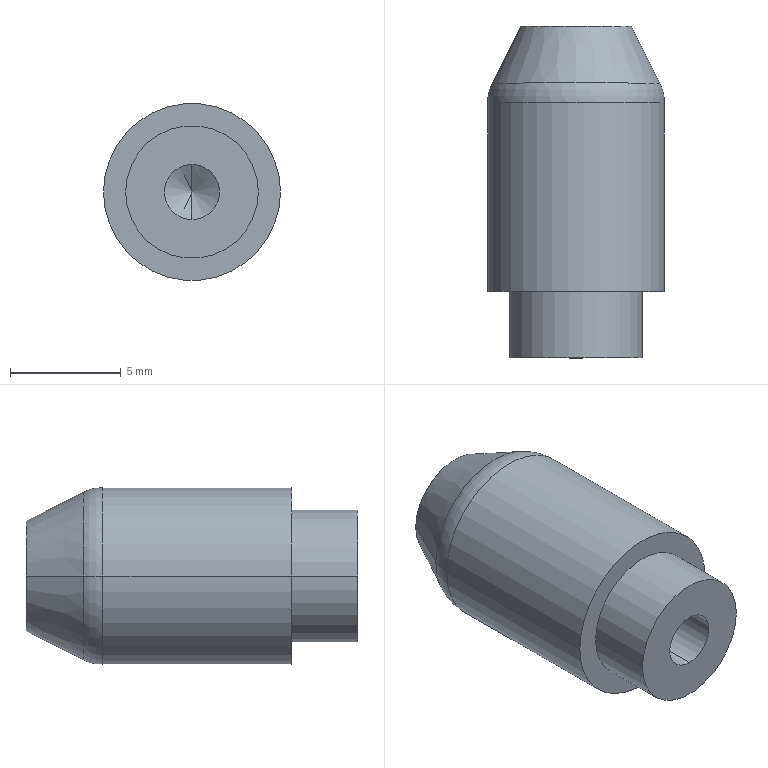Part | SolidWorks | features Fillet 1, HoleWzd 1, Revolution 1 | 1 solid | 15 faces | box 8 x 15 x 8 mm | volume 587.79 mm3 | cylinder 6 | cone 4 | plane 3 | torus 2 | commonest cylinder face diameters 2.5 x2 6 x2 8 x2
STEP:
#1=CARTESIAN_POINT('',(4.,11.528,0.));
#2=VERTEX_POINT('',#1);
#3=CARTESIAN_POINT('',(-4.,11.528,0.));
#4=VERTEX_POINT('',#3);
#5=CARTESIAN_POINT('',(0.,11.528,0.));
#6=DIRECTION('',(0.,-1.,0.));
#7=DIRECTION('',(-1.,0.,0.));
#8=AXIS2_PLACEMENT_3D('',#5,#6,#7);
#9=CIRCLE('',#8,4.);
#10=EDGE_CURVE('',#2,#4,#9,.T.);
#11=ORIENTED_EDGE('',*,*,#10,.F.);
#12=CARTESIAN_POINT('',(3.789,12.422,0.));
#13=VERTEX_POINT('',#12);
#14=CARTESIAN_POINT('',(2.,11.528,0.));
#15=DIRECTION('',(0.,0.,1.));
#16=DIRECTION('',(1.,0.,0.));
#17=AXIS2_PLACEMENT_3D('',#14,#15,#16);
#18=CIRCLE('',#17,2.);
#19=EDGE_CURVE('',#2,#13,#18,.T.);
#20=ORIENTED_EDGE('',*,*,#19,.T.);
#21=CARTESIAN_POINT('',(-3.789,12.422,0.));
#22=VERTEX_POINT('',#21);
#23=CARTESIAN_POINT('',(0.,12.422,0.));
#24=DIRECTION('',(0.,1.,0.));
#25=DIRECTION('',(-1.,0.,0.));
#26=AXIS2_PLACEMENT_3D('',#23,#24,#25);
#27=CIRCLE('',#26,3.789);
#28=EDGE_CURVE('',#22,#13,#27,.T.);
#29=ORIENTED_EDGE('',*,*,#28,.F.);
#30=CARTESIAN_POINT('',(-2.,11.528,0.));
#31=DIRECTION('',(0.,0.,-1.));
#32=DIRECTION('',(-1.,0.,0.));
#33=AXIS2_PLACEMENT_3D('',#30,#31,#32);
#34=CIRCLE('',#33,2.);
#35=EDGE_CURVE('',#4,#22,#34,.T.);
#36=ORIENTED_EDGE('',*,*,#35,.F.);
#37=EDGE_LOOP('',(#11,#20,#29,#36));
#38=FACE_OUTER_BOUND('',#37,.T.);
#39=CARTESIAN_POINT('',(0.,11.528,0.));
#40=DIRECTION('',(0.,1.,0.));
#41=DIRECTION('',(-1.,0.,0.));
#42=AXIS2_PLACEMENT_3D('',#39,#40,#41);
#43=TOROIDAL_SURFACE('',#42,2.,2.);
#44=ADVANCED_FACE('',(#38),#43,.T.);
#45=CARTESIAN_POINT('',(0.,10.,1.25));
#46=VERTEX_POINT('',#45);
#47=CARTESIAN_POINT('',(0.,10.,-1.25));
#48=VERTEX_POINT('',#47);
#49=CARTESIAN_POINT('',(0.,10.,0.));
#50=DIRECTION('',(0.,-1.,0.));
#51=DIRECTION('',(0.,0.,-1.));
#52=AXIS2_PLACEMENT_3D('',#49,#50,#51);
#53=CIRCLE('',#52,1.25);
#54=EDGE_CURVE('',#46,#48,#53,.T.);
#55=ORIENTED_EDGE('',*,*,#54,.F.);
#56=CARTESIAN_POINT('',(0.,0.,1.25));
#57=VERTEX_POINT('',#56);
#58=CARTESIAN_POINT('',(0.,0.,1.25));
#59=DIRECTION('',(0.,-1.,0.));
#60=VECTOR('',#59,1000.);
#61=LINE('',#58,#60);
#62=EDGE_CURVE('',#46,#57,#61,.T.);
#63=ORIENTED_EDGE('',*,*,#62,.T.);
#64=CARTESIAN_POINT('',(0.,0.,-1.25));
#65=VERTEX_POINT('',#64);
#66=CARTESIAN_POINT('',(0.,0.,0.));
#67=DIRECTION('',(0.,-1.,0.));
#68=DIRECTION('',(0.,0.,-1.));
#69=AXIS2_PLACEMENT_3D('',#66,#67,#68);
#70=CIRCLE('',#69,1.25);
#71=EDGE_CURVE('',#57,#65,#70,.T.);
#72=ORIENTED_EDGE('',*,*,#71,.T.);
#73=CARTESIAN_POINT('',(0.,0.,-1.25));
#74=DIRECTION('',(0.,-1.,0.));
#75=VECTOR('',#74,1000.);
#76=LINE('',#73,#75);
#77=EDGE_CURVE('',#48,#65,#76,.T.);
#78=ORIENTED_EDGE('',*,*,#77,.F.);
#79=EDGE_LOOP('',(#55,#63,#72,#78));
#80=FACE_OUTER_BOUND('',#79,.T.);
#81=CARTESIAN_POINT('',(0.,0.,0.));
#82=DIRECTION('',(0.,-1.,0.));
#83=DIRECTION('',(0.,0.,-1.));
#84=AXIS2_PLACEMENT_3D('',#81,#82,#83);
#85=CYLINDRICAL_SURFACE('',#84,1.25);
#86=ADVANCED_FACE('',(#80),#85,.F.);
#87=CARTESIAN_POINT('',(0.,10.751,0.));
#88=VERTEX_POINT('',#87);
#89=CARTESIAN_POINT('',(0.,10.,-1.25));
#90=DIRECTION('',(0.,-0.515,-0.8572));
#91=VECTOR('',#90,1000.);
#92=LINE('',#89,#91);
#93=EDGE_CURVE('',#88,#48,#92,.T.);
#94=ORIENTED_EDGE('',*,*,#93,.F.);
#95=CARTESIAN_POINT('',(0.,10.,1.25));
#96=DIRECTION('',(0.,-0.515,0.8572));
#97=VECTOR('',#96,1000.);
#98=LINE('',#95,#97);
#99=EDGE_CURVE('',#88,#46,#98,.T.);
#100=ORIENTED_EDGE('',*,*,#99,.T.);
#101=ORIENTED_EDGE('',*,*,#54,.T.);
#102=EDGE_LOOP('',(#94,#100,#101));
#103=FACE_OUTER_BOUND('',#102,.T.);
#104=CARTESIAN_POINT('',(0.,10.,0.));
#105=DIRECTION('',(0.,-1.,0.));
#106=DIRECTION('',(0.,0.,-1.));
#107=AXIS2_PLACEMENT_3D('',#104,#105,#106);
#108=CONICAL_SURFACE('',#107,1.25,1.03);
#109=ADVANCED_FACE('',(#103),#108,.F.);
#110=CARTESIAN_POINT('',(3.,3.,0.));
#111=VERTEX_POINT('',#110);
#112=CARTESIAN_POINT('',(-3.,3.,0.));
#113=VERTEX_POINT('',#112);
#114=CARTESIAN_POINT('',(0.,3.,0.));
#115=DIRECTION('',(0.,-1.,0.));
#116=DIRECTION('',(1.,0.,0.));
#117=AXIS2_PLACEMENT_3D('',#114,#115,#116);
#118=CIRCLE('',#117,3.);
#119=EDGE_CURVE('',#111,#113,#118,.T.);
#120=ORIENTED_EDGE('',*,*,#119,.T.);
#121=CARTESIAN_POINT('',(-3.,0.,0.));
#122=VERTEX_POINT('',#121);
#123=CARTESIAN_POINT('',(-3.,0.,0.));
#124=DIRECTION('',(0.,-1.,0.));
#125=VECTOR('',#124,1000.);
#126=LINE('',#123,#125);
#127=EDGE_CURVE('',#113,#122,#126,.T.);
#128=ORIENTED_EDGE('',*,*,#127,.T.);
#129=CARTESIAN_POINT('',(3.,0.,0.));
#130=VERTEX_POINT('',#129);
#131=CARTESIAN_POINT('',(0.,0.,0.));
#132=DIRECTION('',(0.,-1.,0.));
#133=DIRECTION('',(1.,0.,0.));
#134=AXIS2_PLACEMENT_3D('',#131,#132,#133);
#135=CIRCLE('',#134,3.);
#136=EDGE_CURVE('',#130,#122,#135,.T.);
#137=ORIENTED_EDGE('',*,*,#136,.F.);
#138=CARTESIAN_POINT('',(3.,0.,0.));
#139=DIRECTION('',(0.,-1.,0.));
#140=VECTOR('',#139,1000.);
#141=LINE('',#138,#140);
#142=EDGE_CURVE('',#111,#130,#141,.T.);
#143=ORIENTED_EDGE('',*,*,#142,.F.);
#144=EDGE_LOOP('',(#120,#128,#137,#143));
#145=FACE_OUTER_BOUND('',#144,.T.);
#146=CARTESIAN_POINT('',(0.,0.,0.));
#147=DIRECTION('',(0.,-1.,0.));
#148=DIRECTION('',(1.,0.,0.));
#149=AXIS2_PLACEMENT_3D('',#146,#147,#148);
#150=CYLINDRICAL_SURFACE('',#149,3.);
#151=ADVANCED_FACE('',(#145),#150,.T.);
#152=ORIENTED_EDGE('',*,*,#10,.T.);
#153=CARTESIAN_POINT('',(-4.,3.,0.));
#154=VERTEX_POINT('',#153);
#155=CARTESIAN_POINT('',(-4.,0.,0.));
#156=DIRECTION('',(0.,-1.,0.));
#157=VECTOR('',#156,1000.);
#158=LINE('',#155,#157);
#159=EDGE_CURVE('',#4,#154,#158,.T.);
#160=ORIENTED_EDGE('',*,*,#159,.T.);
#161=CARTESIAN_POINT('',(4.,3.,0.));
#162=VERTEX_POINT('',#161);
#163=CARTESIAN_POINT('',(0.,3.,0.));
#164=DIRECTION('',(0.,-1.,0.));
#165=DIRECTION('',(1.,0.,0.));
#166=AXIS2_PLACEMENT_3D('',#163,#164,#165);
#167=CIRCLE('',#166,4.);
#168=EDGE_CURVE('',#162,#154,#167,.T.);
#169=ORIENTED_EDGE('',*,*,#168,.F.);
#170=CARTESIAN_POINT('',(4.,0.,0.));
#171=DIRECTION('',(0.,-1.,0.));
#172=VECTOR('',#171,1000.);
#173=LINE('',#170,#172);
#174=EDGE_CURVE('',#2,#162,#173,.T.);
#175=ORIENTED_EDGE('',*,*,#174,.F.);
#176=EDGE_LOOP('',(#152,#160,#169,#175));
#177=FACE_OUTER_BOUND('',#176,.T.);
#178=CARTESIAN_POINT('',(0.,0.,0.));
#179=DIRECTION('',(0.,-1.,0.));
#180=DIRECTION('',(1.,0.,0.));
#181=AXIS2_PLACEMENT_3D('',#178,#179,#180);
#182=CYLINDRICAL_SURFACE('',#181,4.);
#183=ADVANCED_FACE('',(#177),#182,.T.);
#184=CARTESIAN_POINT('',(2.5,15.,0.));
#185=VERTEX_POINT('',#184);
#186=CARTESIAN_POINT('',(-2.5,15.,0.));
#187=VERTEX_POINT('',#186);
#188=CARTESIAN_POINT('',(0.,15.,0.));
#189=DIRECTION('',(0.,-1.,0.));
#190=DIRECTION('',(1.,0.,0.));
#191=AXIS2_PLACEMENT_3D('',#188,#189,#190);
#192=CIRCLE('',#191,2.5);
#193=EDGE_CURVE('',#185,#187,#192,.T.);
#194=ORIENTED_EDGE('',*,*,#193,.T.);
#195=CARTESIAN_POINT('',(-4.,12.,0.));
#196=DIRECTION('',(-0.4472,-0.8944,0.));
#197=VECTOR('',#196,1000.);
#198=LINE('',#195,#197);
#199=EDGE_CURVE('',#187,#22,#198,.T.);
#200=ORIENTED_EDGE('',*,*,#199,.T.);
#201=ORIENTED_EDGE('',*,*,#28,.T.);
#202=CARTESIAN_POINT('',(4.,12.,0.));
#203=DIRECTION('',(0.4472,-0.8944,0.));
#204=VECTOR('',#203,1000.);
#205=LINE('',#202,#204);
#206=EDGE_CURVE('',#185,#13,#205,.T.);
#207=ORIENTED_EDGE('',*,*,#206,.F.);
#208=EDGE_LOOP('',(#194,#200,#201,#207));
#209=FACE_OUTER_BOUND('',#208,.T.);
#210=CARTESIAN_POINT('',(0.,12.,0.));
#211=DIRECTION('',(0.,-1.,0.));
#212=DIRECTION('',(1.,0.,0.));
#213=AXIS2_PLACEMENT_3D('',#210,#211,#212);
#214=CONICAL_SURFACE('',#213,4.,0.4636);
#215=ADVANCED_FACE('',(#209),#214,.T.);
#216=CARTESIAN_POINT('',(0.,0.,0.));
#217=DIRECTION('',(0.,-1.,0.));
#218=DIRECTION('',(0.,0.,-1.));
#219=AXIS2_PLACEMENT_3D('',#216,#217,#218);
#220=CIRCLE('',#219,1.25);
#221=EDGE_CURVE('',#65,#57,#220,.T.);
#222=ORIENTED_EDGE('',*,*,#221,.F.);
#223=ORIENTED_EDGE('',*,*,#71,.F.);
#224=EDGE_LOOP('',(#222,#223));
#225=FACE_BOUND('',#224,.T.);
#226=ORIENTED_EDGE('',*,*,#136,.T.);
#227=CARTESIAN_POINT('',(0.,0.,0.));
#228=DIRECTION('',(0.,-1.,0.));
#229=DIRECTION('',(1.,0.,0.));
#230=AXIS2_PLACEMENT_3D('',#227,#228,#229);
#231=CIRCLE('',#230,3.);
#232=EDGE_CURVE('',#122,#130,#231,.T.);
#233=ORIENTED_EDGE('',*,*,#232,.T.);
#234=EDGE_LOOP('',(#226,#233));
#235=FACE_OUTER_BOUND('',#234,.T.);
#236=CARTESIAN_POINT('',(3.,0.,0.));
#237=DIRECTION('',(0.,-1.,0.));
#238=DIRECTION('',(1.,0.,0.));
#239=AXIS2_PLACEMENT_3D('',#236,#237,#238);
#240=PLANE('',#239);
#241=ADVANCED_FACE('',(#225,#235),#240,.T.);
#242=ORIENTED_EDGE('',*,*,#193,.F.);
#243=CARTESIAN_POINT('',(0.,15.,0.));
#244=DIRECTION('',(0.,-1.,0.));
#245=DIRECTION('',(1.,0.,0.));
#246=AXIS2_PLACEMENT_3D('',#243,#244,#245);
#247=CIRCLE('',#246,2.5);
#248=EDGE_CURVE('',#187,#185,#247,.T.);
#249=ORIENTED_EDGE('',*,*,#248,.F.);
#250=EDGE_LOOP('',(#242,#249));
#251=FACE_OUTER_BOUND('',#250,.T.);
#252=CARTESIAN_POINT('',(0.,15.,0.));
#253=DIRECTION('',(0.,1.,0.));
#254=DIRECTION('',(-1.,0.,0.));
#255=AXIS2_PLACEMENT_3D('',#252,#253,#254);
#256=PLANE('',#255);
#257=ADVANCED_FACE('',(#251),#256,.T.);
#258=ORIENTED_EDGE('',*,*,#199,.F.);
#259=ORIENTED_EDGE('',*,*,#248,.T.);
#260=ORIENTED_EDGE('',*,*,#206,.T.);
#261=CARTESIAN_POINT('',(0.,12.422,0.));
#262=DIRECTION('',(0.,1.,0.));
#263=DIRECTION('',(-1.,0.,0.));
#264=AXIS2_PLACEMENT_3D('',#261,#262,#263);
#265=CIRCLE('',#264,3.789);
#266=EDGE_CURVE('',#13,#22,#265,.T.);
#267=ORIENTED_EDGE('',*,*,#266,.T.);
#268=EDGE_LOOP('',(#258,#259,#260,#267));
#269=FACE_OUTER_BOUND('',#268,.T.);
#270=CARTESIAN_POINT('',(0.,12.,0.));
#271=DIRECTION('',(0.,-1.,0.));
#272=DIRECTION('',(1.,0.,0.));
#273=AXIS2_PLACEMENT_3D('',#270,#271,#272);
#274=CONICAL_SURFACE('',#273,4.,0.4636);
#275=ADVANCED_FACE('',(#269),#274,.T.);
#276=ORIENTED_EDGE('',*,*,#159,.F.);
#277=CARTESIAN_POINT('',(0.,11.528,0.));
#278=DIRECTION('',(0.,-1.,0.));
#279=DIRECTION('',(-1.,0.,0.));
#280=AXIS2_PLACEMENT_3D('',#277,#278,#279);
#281=CIRCLE('',#280,4.);
#282=EDGE_CURVE('',#4,#2,#281,.T.);
#283=ORIENTED_EDGE('',*,*,#282,.T.);
#284=ORIENTED_EDGE('',*,*,#174,.T.);
#285=CARTESIAN_POINT('',(0.,3.,0.));
#286=DIRECTION('',(0.,-1.,0.));
#287=DIRECTION('',(1.,0.,0.));
#288=AXIS2_PLACEMENT_3D('',#285,#286,#287);
#289=CIRCLE('',#288,4.);
#290=EDGE_CURVE('',#154,#162,#289,.T.);
#291=ORIENTED_EDGE('',*,*,#290,.F.);
#292=EDGE_LOOP('',(#276,#283,#284,#291));
#293=FACE_OUTER_BOUND('',#292,.T.);
#294=CARTESIAN_POINT('',(0.,0.,0.));
#295=DIRECTION('',(0.,-1.,0.));
#296=DIRECTION('',(1.,0.,0.));
#297=AXIS2_PLACEMENT_3D('',#294,#295,#296);
#298=CYLINDRICAL_SURFACE('',#297,4.);
#299=ADVANCED_FACE('',(#293),#298,.T.);
#300=ORIENTED_EDGE('',*,*,#168,.T.);
#301=ORIENTED_EDGE('',*,*,#290,.T.);
#302=EDGE_LOOP('',(#300,#301));
#303=FACE_OUTER_BOUND('',#302,.T.);
#304=ORIENTED_EDGE('',*,*,#119,.F.);
#305=CARTESIAN_POINT('',(0.,3.,0.));
#306=DIRECTION('',(0.,-1.,0.));
#307=DIRECTION('',(1.,0.,0.));
#308=AXIS2_PLACEMENT_3D('',#305,#306,#307);
#309=CIRCLE('',#308,3.);
#310=EDGE_CURVE('',#113,#111,#309,.T.);
#311=ORIENTED_EDGE('',*,*,#310,.F.);
#312=EDGE_LOOP('',(#304,#311));
#313=FACE_BOUND('',#312,.T.);
#314=CARTESIAN_POINT('',(4.,3.,0.));
#315=DIRECTION('',(0.,-1.,0.));
#316=DIRECTION('',(1.,0.,0.));
#317=AXIS2_PLACEMENT_3D('',#314,#315,#316);
#318=PLANE('',#317);
#319=ADVANCED_FACE('',(#303,#313),#318,.T.);
#320=ORIENTED_EDGE('',*,*,#127,.F.);
#321=ORIENTED_EDGE('',*,*,#310,.T.);
#322=ORIENTED_EDGE('',*,*,#142,.T.);
#323=ORIENTED_EDGE('',*,*,#232,.F.);
#324=EDGE_LOOP('',(#320,#321,#322,#323));
#325=FACE_OUTER_BOUND('',#324,.T.);
#326=CARTESIAN_POINT('',(0.,0.,0.));
#327=DIRECTION('',(0.,-1.,0.));
#328=DIRECTION('',(1.,0.,0.));
#329=AXIS2_PLACEMENT_3D('',#326,#327,#328);
#330=CYLINDRICAL_SURFACE('',#329,3.);
#331=ADVANCED_FACE('',(#325),#330,.T.);
#332=ORIENTED_EDGE('',*,*,#99,.F.);
#333=ORIENTED_EDGE('',*,*,#93,.T.);
#334=CARTESIAN_POINT('',(0.,10.,0.));
#335=DIRECTION('',(0.,-1.,0.));
#336=DIRECTION('',(0.,0.,-1.));
#337=AXIS2_PLACEMENT_3D('',#334,#335,#336);
#338=CIRCLE('',#337,1.25);
#339=EDGE_CURVE('',#48,#46,#338,.T.);
#340=ORIENTED_EDGE('',*,*,#339,.T.);
#341=EDGE_LOOP('',(#332,#333,#340));
#342=FACE_OUTER_BOUND('',#341,.T.);
#343=CARTESIAN_POINT('',(0.,10.,0.));
#344=DIRECTION('',(0.,-1.,0.));
#345=DIRECTION('',(0.,0.,-1.));
#346=AXIS2_PLACEMENT_3D('',#343,#344,#345);
#347=CONICAL_SURFACE('',#346,1.25,1.03);
#348=ADVANCED_FACE('',(#342),#347,.F.);
#349=ORIENTED_EDGE('',*,*,#62,.F.);
#350=ORIENTED_EDGE('',*,*,#339,.F.);
#351=ORIENTED_EDGE('',*,*,#77,.T.);
#352=ORIENTED_EDGE('',*,*,#221,.T.);
#353=EDGE_LOOP('',(#349,#350,#351,#352));
#354=FACE_OUTER_BOUND('',#353,.T.);
#355=CARTESIAN_POINT('',(0.,0.,0.));
#356=DIRECTION('',(0.,-1.,0.));
#357=DIRECTION('',(0.,0.,-1.));
#358=AXIS2_PLACEMENT_3D('',#355,#356,#357);
#359=CYLINDRICAL_SURFACE('',#358,1.25);
#360=ADVANCED_FACE('',(#354),#359,.F.);
#361=ORIENTED_EDGE('',*,*,#19,.F.);
#362=ORIENTED_EDGE('',*,*,#282,.F.);
#363=ORIENTED_EDGE('',*,*,#35,.T.);
#364=ORIENTED_EDGE('',*,*,#266,.F.);
#365=EDGE_LOOP('',(#361,#362,#363,#364));
#366=FACE_OUTER_BOUND('',#365,.T.);
#367=CARTESIAN_POINT('',(0.,11.528,0.));
#368=DIRECTION('',(0.,1.,0.));
#369=DIRECTION('',(-1.,0.,0.));
#370=AXIS2_PLACEMENT_3D('',#367,#368,#369);
#371=TOROIDAL_SURFACE('',#370,2.,2.);
#372=ADVANCED_FACE('',(#366),#371,.T.);
#373=CLOSED_SHELL('',(#44,#86,#109,#151,#183,#215,#241,#257,#275,#299,#319,#331,#348,#360,#372));
#374=MANIFOLD_SOLID_BREP('',#373);
#375=CARTESIAN_POINT('',(0.,0.,0.));
#376=DIRECTION('',(0.,0.,1.));
#377=DIRECTION('',(1.,0.,0.));
#378=AXIS2_PLACEMENT_3D('',#375,#376,#377);
#379=(LENGTH_UNIT()NAMED_UNIT(*)SI_UNIT(.MILLI.,.METRE.));
#380=UNCERTAINTY_MEASURE_WITH_UNIT(LENGTH_MEASURE(0.00001),#379,'','');
#381=(NAMED_UNIT(*)PLANE_ANGLE_UNIT()SI_UNIT($,.RADIAN.));
#382=(NAMED_UNIT(*)SI_UNIT($,.STERADIAN.)SOLID_ANGLE_UNIT());
#383=(GEOMETRIC_REPRESENTATION_CONTEXT(3)GLOBAL_UNCERTAINTY_ASSIGNED_CONTEXT((#380))GLOBAL_UNIT_ASSIGNED_CONTEXT((#379,#381,#382))REPRESENTATION_CONTEXT('',''));
#384=ADVANCED_BREP_SHAPE_REPRESENTATION('',(#374,#378),#383);